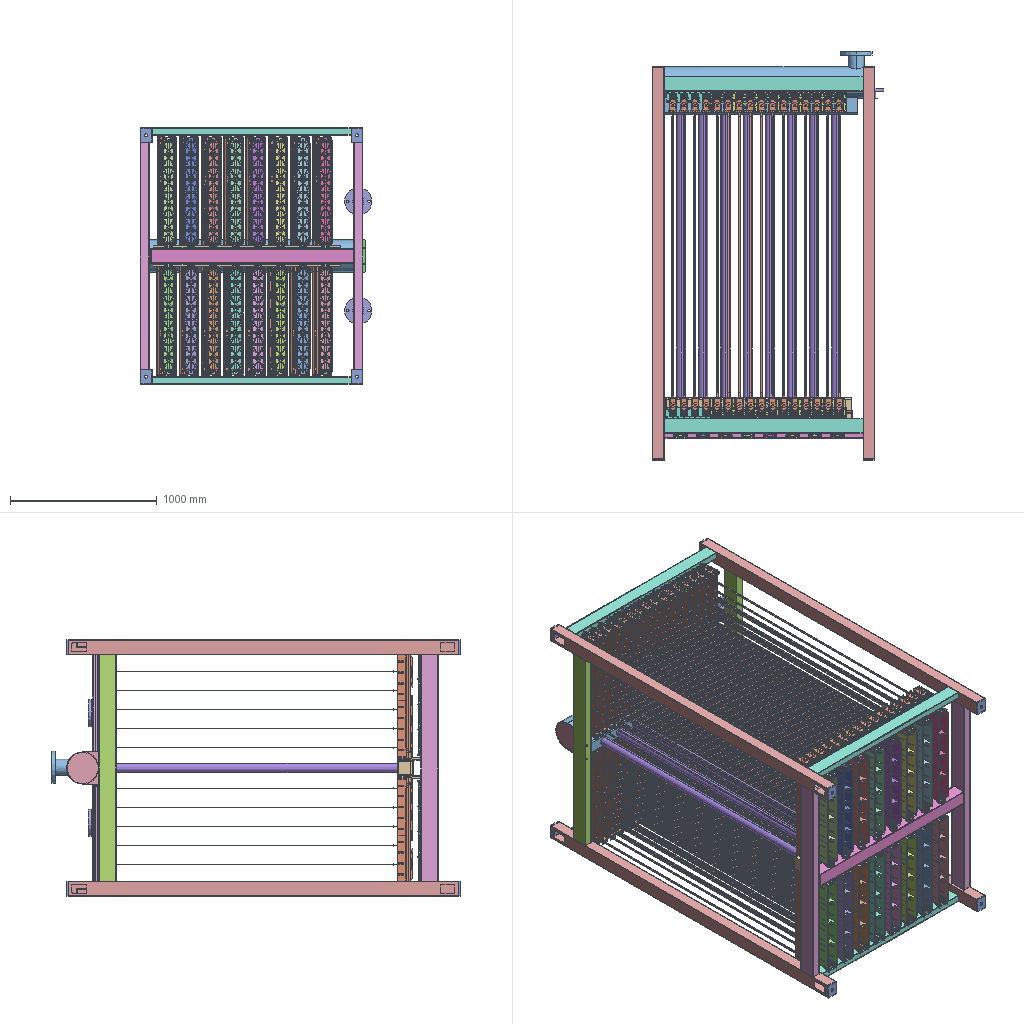Assembly | SolidWorks | 14 different items | 141 placed | box 1577 x 2781 x 1745 mm
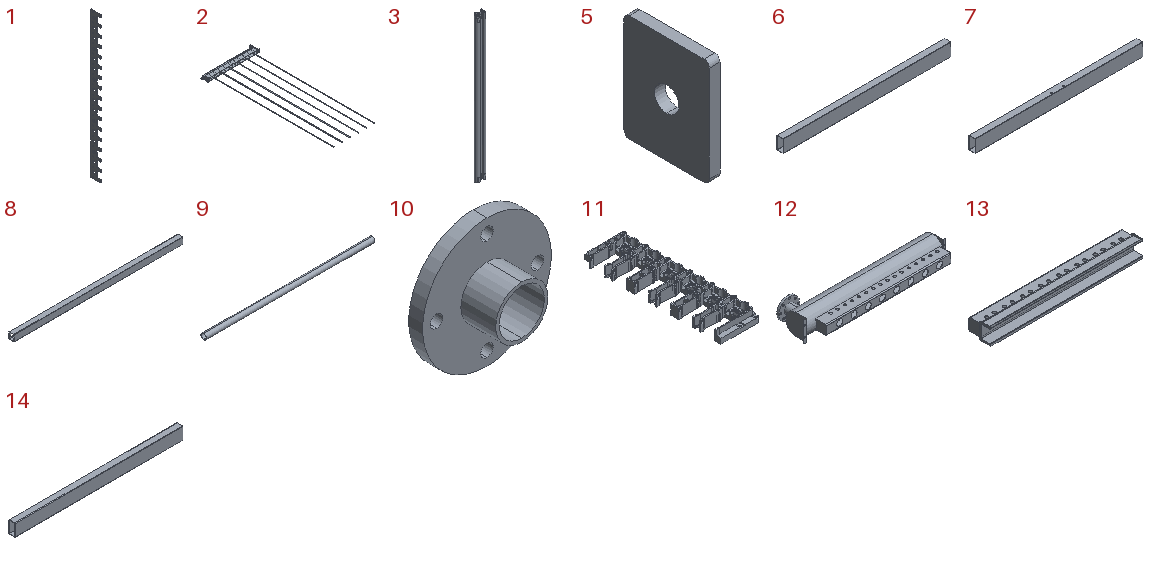Parts list (item | quantity | size | volume | features):
1 | x4 | 4 x 85 x 1231 mm | 272752 mm3 | features BaseBody 1, ICE 1
2 | x64 | 842.8 x 2047 x 56.2 mm | 1758530 mm3 | features BaseBody 2, ICE 1
3 | x32 | 44.505 x 24.701 x 719.001 mm | 253563 mm3 | features BaseBody 1
4 | x1 | - | - | features BaseBody 33, ICE 5
5 | x8 | 10 x 80 x 100 mm | 75631 mm3 | features BaseBody 1
6 | x2 | 1545 x 60 x 120 mm | 1597065 mm3 | features BaseBody 1
7 | x2 | 1545 x 60 x 120 mm | 1595708 mm3 | features BaseBody 1
8 | x4 | 2660 x 80 x 100 mm | 2713722 mm3 | features BaseBody 1
9 | x8 | 1952 x 63 x 63 mm | 1103830 mm3 | features MoveFace 2, BaseBody 1
10 | x2 | 185 x 70 x 185 mm | 505859 mm3 | features ICE 3, Extrusion 1
11 | x8 | 135.78 x 470.75 x 59.95 mm | 480051 mm3 | features BaseBody 1
12 | x1 | 1506 x 424.041 x 224.313 mm | 5157199 mm3 | features ICE 14, BaseBody 3, MoveCopyBody 1, MoveFace 1
13 | x1 | 1272 x 180 x 145 mm | 2844306 mm3 | features ICE 7, BaseBody 3, MoveCopyBody 1
14 | x4 | 1356 x 50 x 100 mm | 1157616 mm3 | features BaseBody 1, MoveFace 1
Mates (type | each side: item.copy, entity, surface, feature):
Coincident | 1.1 face plane Import1 | 11.1 face plane Import1
Concentric | 1.1 face cylinder Import1 | 11.1 face cylinder Import1
Parallel | 1.1 face cylinder Import1 | 11.1 face cylinder Import1
Coincident | 1.2 face plane Import1 | 11.2 face plane Import1
Concentric | 1.2 face cylinder Import1 | 11.2 face cylinder Import1
Parallel | 1.2 face cylinder Import1 | 11.2 face cylinder Import1
Parallel | 14.1 face plane Import1 | 1.2 face plane Import1
Coincident | 8.1 face plane Import1 | 5.1 face plane Import1 | 3 times
Coincident | 8.1 face plane Import1 | 7.1 face plane Import1 | 2 times
Coincident | 8.2 face plane Import1 | 7.1 face plane Import1 | 2 times
Coincident | 8.2 face plane Import1 | 5.2 face plane Import1 | 3 times
Coincident | 8.2 face plane Import1 | 5.3 face plane Import1 | 3 times
Coincident | 8.2 face plane Import1 | 6.1 face plane Import1 | 2 times
Coincident | 8.1 face plane Import1 | 5.4 face plane Import1 | 3 times
Coincident | 8.1 face plane Import1 | 14.2 face plane Import1 | 2 times
Coincident | 5.4 face plane Import1 | 5.5 face plane Import1
Coincident | 6.1 face plane Import1 | 6.2 face plane Import1
Coincident | 7.1 face plane Import1 | 7.2 face plane Import1
Coincident | 7.2 face plane Import1 | 10.1 face plane Boss-Extrude 1
Coincident | 7.2 face plane Import1 | 10.2 face plane Boss-Extrude 1
DistanceDim | 10.2 face cylinder Boss-Extrude 1 | 7.2 face plane Import1
DistanceDim | 10.1 face cylinder Boss-Extrude 1 | 7.2 face plane Import1
DistanceDim | 10.2 face cylinder Boss-Extrude 1 | 8.3 face plane Import1
DistanceDim | 8.4 face plane Import1 | 10.1 face cylinder Boss-Extrude 1
DistanceDim | 5.2 face plane Import1 | 14.3 face plane Import1